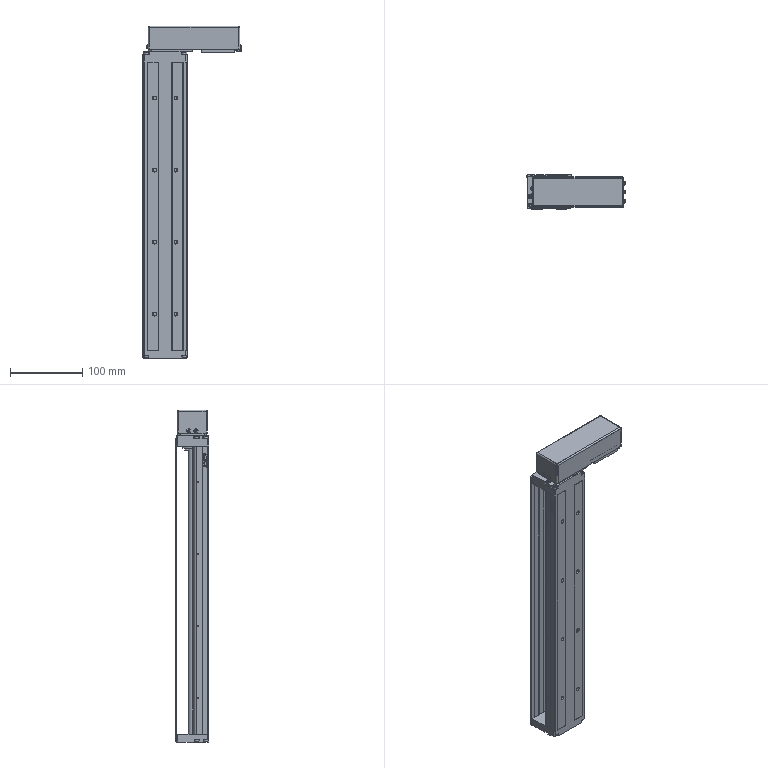Part | SolidWorks | features BaseBody 2 | 2 solids | 976 faces | box 136.45 x 47 x 461 mm | volume 496901 mm3 | plane 557 | cylinder 197 | spline 170 | cone 52 | commonest cylinder face diameters 5.5 x48 2 x18 2.113 x16 2.459 x16 6 x16 9.5 x16